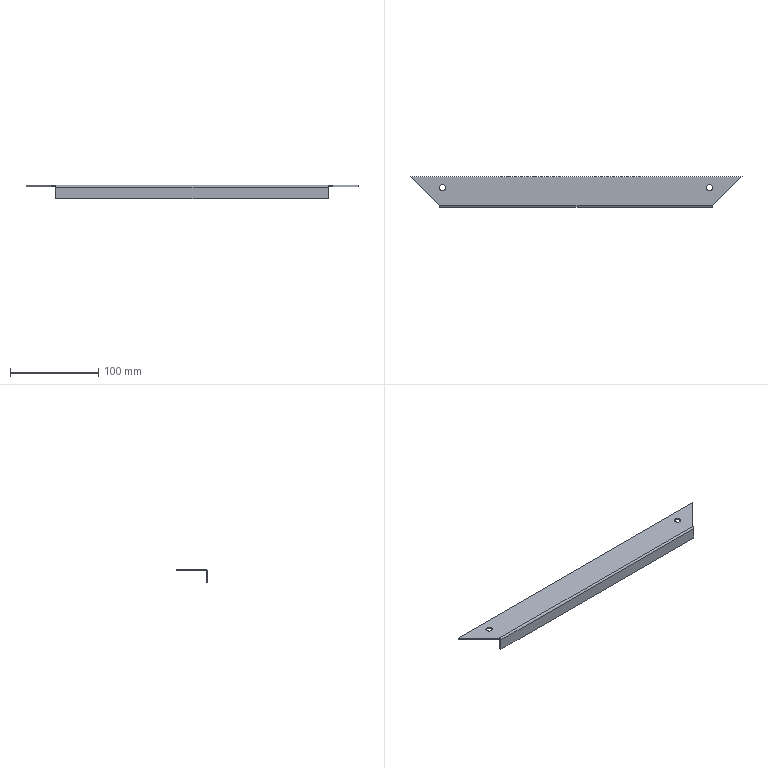Part | STEP file | Right Small Door Clamp Frame 1 | 1 solid | 20 faces | box 376 x 35 x 15 mm | volume 23799 mm3 | plane 12 | cylinder 8 | commonest cylinder face diameters 7 x4 0.15 x2 1 x1 4 x1
STEP:
#1=CARTESIAN_POINT('',(-132.5,257.652,15.));
#2=VERTEX_POINT('',#1);
#3=CARTESIAN_POINT('',(-139.5,257.652,15.));
#4=VERTEX_POINT('',#3);
#5=CARTESIAN_POINT('',(-136.,257.652,15.));
#6=DIRECTION('',(0.,0.,-1.));
#7=DIRECTION('',(-1.,0.,0.));
#8=AXIS2_PLACEMENT_3D('',#5,#6,#7);
#9=CIRCLE('',#8,3.5);
#10=EDGE_CURVE('',#2,#4,#9,.T.);
#11=ORIENTED_EDGE('',*,*,#10,.F.);
#12=CARTESIAN_POINT('',(-132.5,257.652,13.5));
#13=VERTEX_POINT('',#12);
#14=CARTESIAN_POINT('',(-132.5,257.652,15.));
#15=DIRECTION('',(0.,0.,-1.));
#16=VECTOR('',#15,1000.);
#17=LINE('',#14,#16);
#18=EDGE_CURVE('',#2,#13,#17,.T.);
#19=ORIENTED_EDGE('',*,*,#18,.T.);
#20=CARTESIAN_POINT('',(-139.5,257.652,13.5));
#21=VERTEX_POINT('',#20);
#22=CARTESIAN_POINT('',(-136.,257.652,13.5));
#23=DIRECTION('',(0.,0.,-1.));
#24=DIRECTION('',(-1.,0.,0.));
#25=AXIS2_PLACEMENT_3D('',#22,#23,#24);
#26=CIRCLE('',#25,3.5);
#27=EDGE_CURVE('',#13,#21,#26,.T.);
#28=ORIENTED_EDGE('',*,*,#27,.T.);
#29=CARTESIAN_POINT('',(-139.5,257.652,15.));
#30=DIRECTION('',(0.,0.,-1.));
#31=VECTOR('',#30,1000.);
#32=LINE('',#29,#31);
#33=EDGE_CURVE('',#4,#21,#32,.T.);
#34=ORIENTED_EDGE('',*,*,#33,.F.);
#35=EDGE_LOOP('',(#11,#19,#28,#34));
#36=FACE_OUTER_BOUND('',#35,.T.);
#37=CARTESIAN_POINT('',(-136.,257.652,15.));
#38=DIRECTION('',(0.,0.,-1.));
#39=DIRECTION('',(-1.,0.,0.));
#40=AXIS2_PLACEMENT_3D('',#37,#38,#39);
#41=CYLINDRICAL_SURFACE('',#40,3.5);
#42=ADVANCED_FACE('',(#36),#41,.F.);
#43=CARTESIAN_POINT('',(169.5,257.652,15.));
#44=VERTEX_POINT('',#43);
#45=CARTESIAN_POINT('',(162.5,257.652,15.));
#46=VERTEX_POINT('',#45);
#47=CARTESIAN_POINT('',(166.,257.652,15.));
#48=DIRECTION('',(0.,0.,-1.));
#49=DIRECTION('',(-1.,0.,0.));
#50=AXIS2_PLACEMENT_3D('',#47,#48,#49);
#51=CIRCLE('',#50,3.5);
#52=EDGE_CURVE('',#44,#46,#51,.T.);
#53=ORIENTED_EDGE('',*,*,#52,.F.);
#54=CARTESIAN_POINT('',(169.5,257.652,13.5));
#55=VERTEX_POINT('',#54);
#56=CARTESIAN_POINT('',(169.5,257.652,15.));
#57=DIRECTION('',(0.,0.,-1.));
#58=VECTOR('',#57,1000.);
#59=LINE('',#56,#58);
#60=EDGE_CURVE('',#44,#55,#59,.T.);
#61=ORIENTED_EDGE('',*,*,#60,.T.);
#62=CARTESIAN_POINT('',(162.5,257.652,13.5));
#63=VERTEX_POINT('',#62);
#64=CARTESIAN_POINT('',(166.,257.652,13.5));
#65=DIRECTION('',(0.,0.,-1.));
#66=DIRECTION('',(-1.,0.,0.));
#67=AXIS2_PLACEMENT_3D('',#64,#65,#66);
#68=CIRCLE('',#67,3.5);
#69=EDGE_CURVE('',#55,#63,#68,.T.);
#70=ORIENTED_EDGE('',*,*,#69,.T.);
#71=CARTESIAN_POINT('',(162.5,257.652,15.));
#72=DIRECTION('',(0.,0.,-1.));
#73=VECTOR('',#72,1000.);
#74=LINE('',#71,#73);
#75=EDGE_CURVE('',#46,#63,#74,.T.);
#76=ORIENTED_EDGE('',*,*,#75,.F.);
#77=EDGE_LOOP('',(#53,#61,#70,#76));
#78=FACE_OUTER_BOUND('',#77,.T.);
#79=CARTESIAN_POINT('',(166.,257.652,15.));
#80=DIRECTION('',(0.,0.,-1.));
#81=DIRECTION('',(-1.,0.,0.));
#82=AXIS2_PLACEMENT_3D('',#79,#80,#81);
#83=CYLINDRICAL_SURFACE('',#82,3.5);
#84=ADVANCED_FACE('',(#78),#83,.F.);
#85=CARTESIAN_POINT('',(-139.5,237.302,13.5));
#86=VERTEX_POINT('',#85);
#87=CARTESIAN_POINT('',(-139.5,237.152,13.5));
#88=VERTEX_POINT('',#87);
#89=CARTESIAN_POINT('',(-139.5,0.,13.5));
#90=DIRECTION('',(0.,-1.,0.));
#91=VECTOR('',#90,1000.);
#92=LINE('',#89,#91);
#93=EDGE_CURVE('',#86,#88,#92,.T.);
#94=ORIENTED_EDGE('',*,*,#93,.F.);
#95=CARTESIAN_POINT('',(-139.65,237.302,13.5));
#96=VERTEX_POINT('',#95);
#97=CARTESIAN_POINT('',(-139.575,237.302,13.5));
#98=DIRECTION('',(0.,0.,1.));
#99=DIRECTION('',(1.,0.,0.));
#100=AXIS2_PLACEMENT_3D('',#97,#98,#99);
#101=CIRCLE('',#100,0.075);
#102=EDGE_CURVE('',#86,#96,#101,.T.);
#103=ORIENTED_EDGE('',*,*,#102,.T.);
#104=CARTESIAN_POINT('',(-139.65,236.802,13.5));
#105=VERTEX_POINT('',#104);
#106=CARTESIAN_POINT('',(-139.65,0.,13.5));
#107=DIRECTION('',(0.,1.,0.));
#108=VECTOR('',#107,1000.);
#109=LINE('',#106,#108);
#110=EDGE_CURVE('',#105,#96,#109,.T.);
#111=ORIENTED_EDGE('',*,*,#110,.F.);
#112=CARTESIAN_POINT('',(-173.,270.152,13.5));
#113=VERTEX_POINT('',#112);
#114=CARTESIAN_POINT('',(-173.,270.152,13.5));
#115=DIRECTION('',(0.7071,-0.7071,0.));
#116=VECTOR('',#115,1000.);
#117=LINE('',#114,#116);
#118=EDGE_CURVE('',#113,#105,#117,.T.);
#119=ORIENTED_EDGE('',*,*,#118,.F.);
#120=CARTESIAN_POINT('',(203.,270.152,13.5));
#121=VERTEX_POINT('',#120);
#122=CARTESIAN_POINT('',(0.,270.152,13.5));
#123=DIRECTION('',(-1.,0.,0.));
#124=VECTOR('',#123,1000.);
#125=LINE('',#122,#124);
#126=EDGE_CURVE('',#121,#113,#125,.T.);
#127=ORIENTED_EDGE('',*,*,#126,.F.);
#128=CARTESIAN_POINT('',(169.65,236.802,13.5));
#129=VERTEX_POINT('',#128);
#130=CARTESIAN_POINT('',(169.65,236.802,13.5));
#131=DIRECTION('',(0.7071,0.7071,0.));
#132=VECTOR('',#131,1000.);
#133=LINE('',#130,#132);
#134=EDGE_CURVE('',#129,#121,#133,.T.);
#135=ORIENTED_EDGE('',*,*,#134,.F.);
#136=CARTESIAN_POINT('',(169.65,237.302,13.5));
#137=VERTEX_POINT('',#136);
#138=CARTESIAN_POINT('',(169.65,0.,13.5));
#139=DIRECTION('',(0.,-1.,0.));
#140=VECTOR('',#139,1000.);
#141=LINE('',#138,#140);
#142=EDGE_CURVE('',#137,#129,#141,.T.);
#143=ORIENTED_EDGE('',*,*,#142,.F.);
#144=CARTESIAN_POINT('',(169.5,237.302,13.5));
#145=VERTEX_POINT('',#144);
#146=CARTESIAN_POINT('',(169.575,237.302,13.5));
#147=DIRECTION('',(0.,0.,1.));
#148=DIRECTION('',(1.,0.,0.));
#149=AXIS2_PLACEMENT_3D('',#146,#147,#148);
#150=CIRCLE('',#149,0.075);
#151=EDGE_CURVE('',#137,#145,#150,.T.);
#152=ORIENTED_EDGE('',*,*,#151,.T.);
#153=CARTESIAN_POINT('',(169.5,237.152,13.5));
#154=VERTEX_POINT('',#153);
#155=CARTESIAN_POINT('',(169.5,0.,13.5));
#156=DIRECTION('',(0.,1.,0.));
#157=VECTOR('',#156,1000.);
#158=LINE('',#155,#157);
#159=EDGE_CURVE('',#154,#145,#158,.T.);
#160=ORIENTED_EDGE('',*,*,#159,.F.);
#161=CARTESIAN_POINT('',(0.,237.152,13.5));
#162=DIRECTION('',(1.,0.,0.));
#163=VECTOR('',#162,1000.);
#164=LINE('',#161,#163);
#165=EDGE_CURVE('',#88,#154,#164,.T.);
#166=ORIENTED_EDGE('',*,*,#165,.F.);
#167=EDGE_LOOP('',(#94,#103,#111,#119,#127,#135,#143,#152,#160,#166));
#168=FACE_OUTER_BOUND('',#167,.T.);
#169=CARTESIAN_POINT('',(-136.,257.652,13.5));
#170=DIRECTION('',(0.,0.,-1.));
#171=DIRECTION('',(-1.,0.,0.));
#172=AXIS2_PLACEMENT_3D('',#169,#170,#171);
#173=CIRCLE('',#172,3.5);
#174=EDGE_CURVE('',#21,#13,#173,.T.);
#175=ORIENTED_EDGE('',*,*,#174,.F.);
#176=ORIENTED_EDGE('',*,*,#27,.F.);
#177=EDGE_LOOP('',(#175,#176));
#178=FACE_BOUND('',#177,.T.);
#179=CARTESIAN_POINT('',(166.,257.652,13.5));
#180=DIRECTION('',(0.,0.,-1.));
#181=DIRECTION('',(-1.,0.,0.));
#182=AXIS2_PLACEMENT_3D('',#179,#180,#181);
#183=CIRCLE('',#182,3.5);
#184=EDGE_CURVE('',#63,#55,#183,.T.);
#185=ORIENTED_EDGE('',*,*,#184,.F.);
#186=ORIENTED_EDGE('',*,*,#69,.F.);
#187=EDGE_LOOP('',(#185,#186));
#188=FACE_BOUND('',#187,.T.);
#189=CARTESIAN_POINT('',(0.,0.,13.5));
#190=DIRECTION('',(0.,0.,1.));
#191=DIRECTION('',(1.,0.,0.));
#192=AXIS2_PLACEMENT_3D('',#189,#190,#191);
#193=PLANE('',#192);
#194=ADVANCED_FACE('',(#168,#178,#188),#193,.F.);
#195=CARTESIAN_POINT('',(169.5,236.652,13.));
#196=VERTEX_POINT('',#195);
#197=CARTESIAN_POINT('',(169.5,237.152,13.));
#198=DIRECTION('',(-1.,0.,0.));
#199=DIRECTION('',(0.,0.,1.));
#200=AXIS2_PLACEMENT_3D('',#197,#198,#199);
#201=CIRCLE('',#200,0.5);
#202=EDGE_CURVE('',#196,#154,#201,.T.);
#203=ORIENTED_EDGE('',*,*,#202,.F.);
#204=CARTESIAN_POINT('',(-139.5,236.652,13.));
#205=VERTEX_POINT('',#204);
#206=CARTESIAN_POINT('',(548.511,236.652,13.));
#207=DIRECTION('',(1.,0.,0.));
#208=VECTOR('',#207,1000.);
#209=LINE('',#206,#208);
#210=EDGE_CURVE('',#205,#196,#209,.T.);
#211=ORIENTED_EDGE('',*,*,#210,.F.);
#212=CARTESIAN_POINT('',(-139.5,237.152,13.));
#213=DIRECTION('',(1.,0.,0.));
#214=DIRECTION('',(0.,0.,1.));
#215=AXIS2_PLACEMENT_3D('',#212,#213,#214);
#216=CIRCLE('',#215,0.5);
#217=EDGE_CURVE('',#88,#205,#216,.T.);
#218=ORIENTED_EDGE('',*,*,#217,.F.);
#219=ORIENTED_EDGE('',*,*,#165,.T.);
#220=EDGE_LOOP('',(#203,#211,#218,#219));
#221=FACE_OUTER_BOUND('',#220,.T.);
#222=CARTESIAN_POINT('',(548.511,237.152,13.));
#223=DIRECTION('',(-1.,0.,0.));
#224=DIRECTION('',(0.,0.,1.));
#225=AXIS2_PLACEMENT_3D('',#222,#223,#224);
#226=CYLINDRICAL_SURFACE('',#225,0.5);
#227=ADVANCED_FACE('',(#221),#226,.F.);
#228=CARTESIAN_POINT('',(-173.,270.152,15.));
#229=VERTEX_POINT('',#228);
#230=CARTESIAN_POINT('',(-173.,270.152,-739.952));
#231=DIRECTION('',(0.,0.,-1.));
#232=VECTOR('',#231,1000.);
#233=LINE('',#230,#232);
#234=EDGE_CURVE('',#229,#113,#233,.T.);
#235=ORIENTED_EDGE('',*,*,#234,.T.);
#236=ORIENTED_EDGE('',*,*,#118,.T.);
#237=CARTESIAN_POINT('',(-139.65,236.802,15.));
#238=VERTEX_POINT('',#237);
#239=CARTESIAN_POINT('',(-139.65,236.802,-739.952));
#240=DIRECTION('',(0.,0.,1.));
#241=VECTOR('',#240,1000.);
#242=LINE('',#239,#241);
#243=EDGE_CURVE('',#105,#238,#242,.T.);
#244=ORIENTED_EDGE('',*,*,#243,.T.);
#245=CARTESIAN_POINT('',(48.576,48.576,15.));
#246=DIRECTION('',(-0.7071,0.7071,0.));
#247=VECTOR('',#246,1000.);
#248=LINE('',#245,#247);
#249=EDGE_CURVE('',#238,#229,#248,.T.);
#250=ORIENTED_EDGE('',*,*,#249,.T.);
#251=EDGE_LOOP('',(#235,#236,#244,#250));
#252=FACE_OUTER_BOUND('',#251,.T.);
#253=CARTESIAN_POINT('',(48.576,48.576,-739.952));
#254=DIRECTION('',(-0.7071,-0.7071,0.));
#255=DIRECTION('',(0.7071,-0.7071,0.));
#256=AXIS2_PLACEMENT_3D('',#253,#254,#255);
#257=PLANE('',#256);
#258=ADVANCED_FACE('',(#252),#257,.T.);
#259=CARTESIAN_POINT('',(203.,270.152,15.));
#260=VERTEX_POINT('',#259);
#261=CARTESIAN_POINT('',(203.,270.152,-739.952));
#262=DIRECTION('',(0.,0.,-1.));
#263=VECTOR('',#262,1000.);
#264=LINE('',#261,#263);
#265=EDGE_CURVE('',#260,#121,#264,.T.);
#266=ORIENTED_EDGE('',*,*,#265,.T.);
#267=ORIENTED_EDGE('',*,*,#126,.T.);
#268=ORIENTED_EDGE('',*,*,#234,.F.);
#269=CARTESIAN_POINT('',(-173.,270.152,15.));
#270=DIRECTION('',(1.,0.,0.));
#271=VECTOR('',#270,1000.);
#272=LINE('',#269,#271);
#273=EDGE_CURVE('',#229,#260,#272,.T.);
#274=ORIENTED_EDGE('',*,*,#273,.T.);
#275=EDGE_LOOP('',(#266,#267,#268,#274));
#276=FACE_OUTER_BOUND('',#275,.T.);
#277=CARTESIAN_POINT('',(-173.,270.152,-739.952));
#278=DIRECTION('',(0.,1.,0.));
#279=DIRECTION('',(0.,0.,1.));
#280=AXIS2_PLACEMENT_3D('',#277,#278,#279);
#281=PLANE('',#280);
#282=ADVANCED_FACE('',(#276),#281,.T.);
#283=CARTESIAN_POINT('',(169.65,236.802,15.));
#284=VERTEX_POINT('',#283);
#285=CARTESIAN_POINT('',(169.65,236.802,-739.952));
#286=DIRECTION('',(0.,0.,-1.));
#287=VECTOR('',#286,1000.);
#288=LINE('',#285,#287);
#289=EDGE_CURVE('',#284,#129,#288,.T.);
#290=ORIENTED_EDGE('',*,*,#289,.T.);
#291=ORIENTED_EDGE('',*,*,#134,.T.);
#292=ORIENTED_EDGE('',*,*,#265,.F.);
#293=CARTESIAN_POINT('',(-33.576,33.576,15.));
#294=DIRECTION('',(-0.7071,-0.7071,0.));
#295=VECTOR('',#294,1000.);
#296=LINE('',#293,#295);
#297=EDGE_CURVE('',#260,#284,#296,.T.);
#298=ORIENTED_EDGE('',*,*,#297,.T.);
#299=EDGE_LOOP('',(#290,#291,#292,#298));
#300=FACE_OUTER_BOUND('',#299,.T.);
#301=CARTESIAN_POINT('',(-33.576,33.576,-739.952));
#302=DIRECTION('',(0.7071,-0.7071,0.));
#303=DIRECTION('',(0.7071,0.7071,0.));
#304=AXIS2_PLACEMENT_3D('',#301,#302,#303);
#305=PLANE('',#304);
#306=ADVANCED_FACE('',(#300),#305,.T.);
#307=ORIENTED_EDGE('',*,*,#18,.F.);
#308=CARTESIAN_POINT('',(-136.,257.652,15.));
#309=DIRECTION('',(0.,0.,-1.));
#310=DIRECTION('',(-1.,0.,0.));
#311=AXIS2_PLACEMENT_3D('',#308,#309,#310);
#312=CIRCLE('',#311,3.5);
#313=EDGE_CURVE('',#4,#2,#312,.T.);
#314=ORIENTED_EDGE('',*,*,#313,.F.);
#315=ORIENTED_EDGE('',*,*,#33,.T.);
#316=ORIENTED_EDGE('',*,*,#174,.T.);
#317=EDGE_LOOP('',(#307,#314,#315,#316));
#318=FACE_OUTER_BOUND('',#317,.T.);
#319=CARTESIAN_POINT('',(-136.,257.652,15.));
#320=DIRECTION('',(0.,0.,-1.));
#321=DIRECTION('',(-1.,0.,0.));
#322=AXIS2_PLACEMENT_3D('',#319,#320,#321);
#323=CYLINDRICAL_SURFACE('',#322,3.5);
#324=ADVANCED_FACE('',(#318),#323,.F.);
#325=ORIENTED_EDGE('',*,*,#60,.F.);
#326=CARTESIAN_POINT('',(166.,257.652,15.));
#327=DIRECTION('',(0.,0.,-1.));
#328=DIRECTION('',(-1.,0.,0.));
#329=AXIS2_PLACEMENT_3D('',#326,#327,#328);
#330=CIRCLE('',#329,3.5);
#331=EDGE_CURVE('',#46,#44,#330,.T.);
#332=ORIENTED_EDGE('',*,*,#331,.F.);
#333=ORIENTED_EDGE('',*,*,#75,.T.);
#334=ORIENTED_EDGE('',*,*,#184,.T.);
#335=EDGE_LOOP('',(#325,#332,#333,#334));
#336=FACE_OUTER_BOUND('',#335,.T.);
#337=CARTESIAN_POINT('',(166.,257.652,15.));
#338=DIRECTION('',(0.,0.,-1.));
#339=DIRECTION('',(-1.,0.,0.));
#340=AXIS2_PLACEMENT_3D('',#337,#338,#339);
#341=CYLINDRICAL_SURFACE('',#340,3.5);
#342=ADVANCED_FACE('',(#336),#341,.F.);
#343=ORIENTED_EDGE('',*,*,#210,.T.);
#344=CARTESIAN_POINT('',(169.5,236.652,0.));
#345=VERTEX_POINT('',#344);
#346=CARTESIAN_POINT('',(169.5,236.652,15.));
#347=DIRECTION('',(0.,0.,1.));
#348=VECTOR('',#347,1000.);
#349=LINE('',#346,#348);
#350=EDGE_CURVE('',#345,#196,#349,.T.);
#351=ORIENTED_EDGE('',*,*,#350,.F.);
#352=CARTESIAN_POINT('',(-139.5,236.652,0.));
#353=VERTEX_POINT('',#352);
#354=CARTESIAN_POINT('',(-138.,236.652,0.));
#355=DIRECTION('',(1.,0.,0.));
#356=VECTOR('',#355,1000.);
#357=LINE('',#354,#356);
#358=EDGE_CURVE('',#353,#345,#357,.T.);
#359=ORIENTED_EDGE('',*,*,#358,.F.);
#360=CARTESIAN_POINT('',(-139.5,236.652,15.));
#361=DIRECTION('',(0.,0.,-1.));
#362=VECTOR('',#361,1000.);
#363=LINE('',#360,#362);
#364=EDGE_CURVE('',#205,#353,#363,.T.);
#365=ORIENTED_EDGE('',*,*,#364,.F.);
#366=EDGE_LOOP('',(#343,#351,#359,#365));
#367=FACE_OUTER_BOUND('',#366,.T.);
#368=CARTESIAN_POINT('',(-138.,236.652,15.));
#369=DIRECTION('',(0.,-1.,0.));
#370=DIRECTION('',(0.,0.,-1.));
#371=AXIS2_PLACEMENT_3D('',#368,#369,#370);
#372=PLANE('',#371);
#373=ADVANCED_FACE('',(#367),#372,.F.);
#374=CARTESIAN_POINT('',(-139.65,237.302,15.));
#375=VERTEX_POINT('',#374);
#376=CARTESIAN_POINT('',(-139.65,0.,15.));
#377=DIRECTION('',(0.,1.,0.));
#378=VECTOR('',#377,1000.);
#379=LINE('',#376,#378);
#380=EDGE_CURVE('',#238,#375,#379,.T.);
#381=ORIENTED_EDGE('',*,*,#380,.T.);
#382=CARTESIAN_POINT('',(-139.5,237.302,15.));
#383=VERTEX_POINT('',#382);
#384=CARTESIAN_POINT('',(-139.575,237.302,15.));
#385=DIRECTION('',(0.,0.,-1.));
#386=DIRECTION('',(1.,0.,0.));
#387=AXIS2_PLACEMENT_3D('',#384,#385,#386);
#388=CIRCLE('',#387,0.075);
#389=EDGE_CURVE('',#375,#383,#388,.T.);
#390=ORIENTED_EDGE('',*,*,#389,.T.);
#391=CARTESIAN_POINT('',(-139.5,237.152,15.));
#392=VERTEX_POINT('',#391);
#393=CARTESIAN_POINT('',(-139.5,0.,15.));
#394=DIRECTION('',(0.,1.,0.));
#395=VECTOR('',#394,1000.);
#396=LINE('',#393,#395);
#397=EDGE_CURVE('',#392,#383,#396,.T.);
#398=ORIENTED_EDGE('',*,*,#397,.F.);
#399=CARTESIAN_POINT('',(169.5,237.152,15.));
#400=VERTEX_POINT('',#399);
#401=CARTESIAN_POINT('',(0.,237.152,15.));
#402=DIRECTION('',(1.,0.,0.));
#403=VECTOR('',#402,1000.);
#404=LINE('',#401,#403);
#405=EDGE_CURVE('',#392,#400,#404,.T.);
#406=ORIENTED_EDGE('',*,*,#405,.T.);
#407=CARTESIAN_POINT('',(169.5,237.302,15.));
#408=VERTEX_POINT('',#407);
#409=CARTESIAN_POINT('',(169.5,0.,15.));
#410=DIRECTION('',(0.,-1.,0.));
#411=VECTOR('',#410,1000.);
#412=LINE('',#409,#411);
#413=EDGE_CURVE('',#408,#400,#412,.T.);
#414=ORIENTED_EDGE('',*,*,#413,.F.);
#415=CARTESIAN_POINT('',(169.65,237.302,15.));
#416=VERTEX_POINT('',#415);
#417=CARTESIAN_POINT('',(169.575,237.302,15.));
#418=DIRECTION('',(0.,0.,-1.));
#419=DIRECTION('',(1.,0.,0.));
#420=AXIS2_PLACEMENT_3D('',#417,#418,#419);
#421=CIRCLE('',#420,0.075);
#422=EDGE_CURVE('',#408,#416,#421,.T.);
#423=ORIENTED_EDGE('',*,*,#422,.T.);
#424=CARTESIAN_POINT('',(169.65,0.,15.));
#425=DIRECTION('',(0.,-1.,0.));
#426=VECTOR('',#425,1000.);
#427=LINE('',#424,#426);
#428=EDGE_CURVE('',#416,#284,#427,.T.);
#429=ORIENTED_EDGE('',*,*,#428,.T.);
#430=ORIENTED_EDGE('',*,*,#297,.F.);
#431=ORIENTED_EDGE('',*,*,#273,.F.);
#432=ORIENTED_EDGE('',*,*,#249,.F.);
#433=EDGE_LOOP('',(#381,#390,#398,#406,#414,#423,#429,#430,#431,#432));
#434=FACE_OUTER_BOUND('',#433,.T.);
#435=ORIENTED_EDGE('',*,*,#313,.T.);
#436=ORIENTED_EDGE('',*,*,#10,.T.);
#437=EDGE_LOOP('',(#435,#436));
#438=FACE_BOUND('',#437,.T.);
#439=ORIENTED_EDGE('',*,*,#331,.T.);
#440=ORIENTED_EDGE('',*,*,#52,.T.);
#441=EDGE_LOOP('',(#439,#440));
#442=FACE_BOUND('',#441,.T.);
#443=CARTESIAN_POINT('',(0.,0.,15.));
#444=DIRECTION('',(0.,0.,1.));
#445=DIRECTION('',(1.,0.,0.));
#446=AXIS2_PLACEMENT_3D('',#443,#444,#445);
#447=PLANE('',#446);
#448=ADVANCED_FACE('',(#434,#438,#442),#447,.T.);
#449=ORIENTED_EDGE('',*,*,#243,.F.);
#450=ORIENTED_EDGE('',*,*,#110,.T.);
#451=CARTESIAN_POINT('',(-139.65,237.302,-739.952));
#452=DIRECTION('',(0.,0.,1.));
#453=VECTOR('',#452,1000.);
#454=LINE('',#451,#453);
#455=EDGE_CURVE('',#96,#375,#454,.T.);
#456=ORIENTED_EDGE('',*,*,#455,.T.);
#457=ORIENTED_EDGE('',*,*,#380,.F.);
#458=EDGE_LOOP('',(#449,#450,#456,#457));
#459=FACE_OUTER_BOUND('',#458,.T.);
#460=CARTESIAN_POINT('',(-139.65,0.,-739.952));
#461=DIRECTION('',(1.,0.,0.));
#462=DIRECTION('',(0.,0.,-1.));
#463=AXIS2_PLACEMENT_3D('',#460,#461,#462);
#464=PLANE('',#463);
#465=ADVANCED_FACE('',(#459),#464,.T.);
#466=CARTESIAN_POINT('',(169.65,237.302,-739.952));
#467=DIRECTION('',(0.,0.,-1.));
#468=VECTOR('',#467,1000.);
#469=LINE('',#466,#468);
#470=EDGE_CURVE('',#416,#137,#469,.T.);
#471=ORIENTED_EDGE('',*,*,#470,.T.);
#472=ORIENTED_EDGE('',*,*,#142,.T.);
#473=ORIENTED_EDGE('',*,*,#289,.F.);
#474=ORIENTED_EDGE('',*,*,#428,.F.);
#475=EDGE_LOOP('',(#471,#472,#473,#474));
#476=FACE_OUTER_BOUND('',#475,.T.);
#477=CARTESIAN_POINT('',(169.65,0.,-739.952));
#478=DIRECTION('',(-1.,0.,0.));
#479=DIRECTION('',(0.,0.,1.));
#480=AXIS2_PLACEMENT_3D('',#477,#478,#479);
#481=PLANE('',#480);
#482=ADVANCED_FACE('',(#476),#481,.T.);
#483=CARTESIAN_POINT('',(-139.5,235.152,0.));
#484=VERTEX_POINT('',#483);
#485=CARTESIAN_POINT('',(-139.5,235.152,13.));
#486=VERTEX_POINT('',#485);
#487=CARTESIAN_POINT('',(-139.5,235.152,15.));
#488=DIRECTION('',(0.,0.,1.));
#489=VECTOR('',#488,1000.);
#490=LINE('',#487,#489);
#491=EDGE_CURVE('',#484,#486,#490,.T.);
#492=ORIENTED_EDGE('',*,*,#491,.T.);
#493=CARTESIAN_POINT('',(-139.5,237.152,13.));
#494=DIRECTION('',(1.,0.,0.));
#495=DIRECTION('',(0.,0.,1.));
#496=AXIS2_PLACEMENT_3D('',#493,#494,#495);
#497=CIRCLE('',#496,2.);
#498=EDGE_CURVE('',#392,#486,#497,.T.);
#499=ORIENTED_EDGE('',*,*,#498,.F.);
#500=ORIENTED_EDGE('',*,*,#397,.T.);
#501=CARTESIAN_POINT('',(-139.5,237.302,-739.952));
#502=DIRECTION('',(0.,0.,-1.));
#503=VECTOR('',#502,1000.);
#504=LINE('',#501,#503);
#505=EDGE_CURVE('',#383,#86,#504,.T.);
#506=ORIENTED_EDGE('',*,*,#505,.T.);
#507=ORIENTED_EDGE('',*,*,#93,.T.);
#508=ORIENTED_EDGE('',*,*,#217,.T.);
#509=ORIENTED_EDGE('',*,*,#364,.T.);
#510=CARTESIAN_POINT('',(-139.5,853.699,0.));
#511=DIRECTION('',(0.,-1.,0.));
#512=VECTOR('',#511,1000.);
#513=LINE('',#510,#512);
#514=EDGE_CURVE('',#353,#484,#513,.T.);
#515=ORIENTED_EDGE('',*,*,#514,.T.);
#516=EDGE_LOOP('',(#492,#499,#500,#506,#507,#508,#509,#515));
#517=FACE_OUTER_BOUND('',#516,.T.);
#518=CARTESIAN_POINT('',(-139.5,853.699,15.));
#519=DIRECTION('',(-1.,0.,0.));
#520=DIRECTION('',(0.,0.,1.));
#521=AXIS2_PLACEMENT_3D('',#518,#519,#520);
#522=PLANE('',#521);
#523=ADVANCED_FACE('',(#517),#522,.T.);
#524=CARTESIAN_POINT('',(169.5,235.152,0.));
#525=VERTEX_POINT('',#524);
#526=CARTESIAN_POINT('',(169.5,853.699,0.));
#527=DIRECTION('',(0.,-1.,0.));
#528=VECTOR('',#527,1000.);
#529=LINE('',#526,#528);
#530=EDGE_CURVE('',#345,#525,#529,.T.);
#531=ORIENTED_EDGE('',*,*,#530,.F.);
#532=ORIENTED_EDGE('',*,*,#350,.T.);
#533=ORIENTED_EDGE('',*,*,#202,.T.);
#534=ORIENTED_EDGE('',*,*,#159,.T.);
#535=CARTESIAN_POINT('',(169.5,237.302,-739.952));
#536=DIRECTION('',(0.,0.,1.));
#537=VECTOR('',#536,1000.);
#538=LINE('',#535,#537);
#539=EDGE_CURVE('',#145,#408,#538,.T.);
#540=ORIENTED_EDGE('',*,*,#539,.T.);
#541=ORIENTED_EDGE('',*,*,#413,.T.);
#542=CARTESIAN_POINT('',(169.5,235.152,13.));
#543=VERTEX_POINT('',#542);
#544=CARTESIAN_POINT('',(169.5,237.152,13.));
#545=DIRECTION('',(-1.,0.,0.));
#546=DIRECTION('',(0.,0.,1.));
#547=AXIS2_PLACEMENT_3D('',#544,#545,#546);
#548=CIRCLE('',#547,2.);
#549=EDGE_CURVE('',#543,#400,#548,.T.);
#550=ORIENTED_EDGE('',*,*,#549,.F.);
#551=CARTESIAN_POINT('',(169.5,235.152,15.));
#552=DIRECTION('',(0.,0.,1.));
#553=VECTOR('',#552,1000.);
#554=LINE('',#551,#553);
#555=EDGE_CURVE('',#525,#543,#554,.T.);
#556=ORIENTED_EDGE('',*,*,#555,.F.);
#557=EDGE_LOOP('',(#531,#532,#533,#534,#540,#541,#550,#556));
#558=FACE_OUTER_BOUND('',#557,.T.);
#559=CARTESIAN_POINT('',(169.5,853.699,15.));
#560=DIRECTION('',(-1.,0.,0.));
#561=DIRECTION('',(0.,0.,1.));
#562=AXIS2_PLACEMENT_3D('',#559,#560,#561);
#563=PLANE('',#562);
#564=ADVANCED_FACE('',(#558),#563,.F.);
#565=ORIENTED_EDGE('',*,*,#514,.F.);
#566=ORIENTED_EDGE('',*,*,#358,.T.);
#567=ORIENTED_EDGE('',*,*,#530,.T.);
#568=CARTESIAN_POINT('',(-138.,235.152,0.));
#569=DIRECTION('',(1.,0.,0.));
#570=VECTOR('',#569,1000.);
#571=LINE('',#568,#570);
#572=EDGE_CURVE('',#484,#525,#571,.T.);
#573=ORIENTED_EDGE('',*,*,#572,.F.);
#574=EDGE_LOOP('',(#565,#566,#567,#573));
#575=FACE_OUTER_BOUND('',#574,.T.);
#576=CARTESIAN_POINT('',(-138.,853.699,0.));
#577=DIRECTION('',(0.,0.,1.));
#578=DIRECTION('',(0.,-1.,0.));
#579=AXIS2_PLACEMENT_3D('',#576,#577,#578);
#580=PLANE('',#579);
#581=ADVANCED_FACE('',(#575),#580,.F.);
#582=CARTESIAN_POINT('',(548.511,235.152,13.));
#583=DIRECTION('',(1.,0.,0.));
#584=VECTOR('',#583,1000.);
#585=LINE('',#582,#584);
#586=EDGE_CURVE('',#486,#543,#585,.T.);
#587=ORIENTED_EDGE('',*,*,#586,.T.);
#588=ORIENTED_EDGE('',*,*,#549,.T.);
#589=ORIENTED_EDGE('',*,*,#405,.F.);
#590=ORIENTED_EDGE('',*,*,#498,.T.);
#591=EDGE_LOOP('',(#587,#588,#589,#590));
#592=FACE_OUTER_BOUND('',#591,.T.);
#593=CARTESIAN_POINT('',(548.511,237.152,13.));
#594=DIRECTION('',(-1.,0.,0.));
#595=DIRECTION('',(0.,0.,1.));
#596=AXIS2_PLACEMENT_3D('',#593,#594,#595);
#597=CYLINDRICAL_SURFACE('',#596,2.);
#598=ADVANCED_FACE('',(#592),#597,.T.);
#599=ORIENTED_EDGE('',*,*,#455,.F.);
#600=ORIENTED_EDGE('',*,*,#102,.F.);
#601=ORIENTED_EDGE('',*,*,#505,.F.);
#602=ORIENTED_EDGE('',*,*,#389,.F.);
#603=EDGE_LOOP('',(#599,#600,#601,#602));
#604=FACE_OUTER_BOUND('',#603,.T.);
#605=CARTESIAN_POINT('',(-139.575,237.302,-739.952));
#606=DIRECTION('',(0.,0.,1.));
#607=DIRECTION('',(1.,0.,0.));
#608=AXIS2_PLACEMENT_3D('',#605,#606,#607);
#609=CYLINDRICAL_SURFACE('',#608,0.075);
#610=ADVANCED_FACE('',(#604),#609,.F.);
#611=ORIENTED_EDGE('',*,*,#539,.F.);
#612=ORIENTED_EDGE('',*,*,#151,.F.);
#613=ORIENTED_EDGE('',*,*,#470,.F.);
#614=ORIENTED_EDGE('',*,*,#422,.F.);
#615=EDGE_LOOP('',(#611,#612,#613,#614));
#616=FACE_OUTER_BOUND('',#615,.T.);
#617=CARTESIAN_POINT('',(169.575,237.302,-739.952));
#618=DIRECTION('',(0.,0.,1.));
#619=DIRECTION('',(1.,0.,0.));
#620=AXIS2_PLACEMENT_3D('',#617,#618,#619);
#621=CYLINDRICAL_SURFACE('',#620,0.075);
#622=ADVANCED_FACE('',(#616),#621,.F.);
#623=ORIENTED_EDGE('',*,*,#572,.T.);
#624=ORIENTED_EDGE('',*,*,#555,.T.);
#625=ORIENTED_EDGE('',*,*,#586,.F.);
#626=ORIENTED_EDGE('',*,*,#491,.F.);
#627=EDGE_LOOP('',(#623,#624,#625,#626));
#628=FACE_OUTER_BOUND('',#627,.T.);
#629=CARTESIAN_POINT('',(-138.,235.152,15.));
#630=DIRECTION('',(0.,-1.,0.));
#631=DIRECTION('',(0.,0.,-1.));
#632=AXIS2_PLACEMENT_3D('',#629,#630,#631);
#633=PLANE('',#632);
#634=ADVANCED_FACE('',(#628),#633,.T.);
#635=CLOSED_SHELL('',(#42,#84,#194,#227,#258,#282,#306,#324,#342,#373,#448,#465,#482,#523,#564,#581,#598,#610,#622,#634));
#636=MANIFOLD_SOLID_BREP('',#635);
#637=CARTESIAN_POINT('',(0.,0.,0.));
#638=DIRECTION('',(0.,0.,1.));
#639=DIRECTION('',(1.,0.,0.));
#640=AXIS2_PLACEMENT_3D('',#637,#638,#639);
#641=(LENGTH_UNIT()NAMED_UNIT(*)SI_UNIT(.MILLI.,.METRE.));
#642=UNCERTAINTY_MEASURE_WITH_UNIT(LENGTH_MEASURE(0.00001),#641,'','');
#643=(NAMED_UNIT(*)PLANE_ANGLE_UNIT()SI_UNIT($,.RADIAN.));
#644=(NAMED_UNIT(*)SI_UNIT($,.STERADIAN.)SOLID_ANGLE_UNIT());
#645=(GEOMETRIC_REPRESENTATION_CONTEXT(3)GLOBAL_UNCERTAINTY_ASSIGNED_CONTEXT((#642))GLOBAL_UNIT_ASSIGNED_CONTEXT((#641,#643,#644))REPRESENTATION_CONTEXT('',''));
#646=ADVANCED_BREP_SHAPE_REPRESENTATION('',(#636,#640),#645);